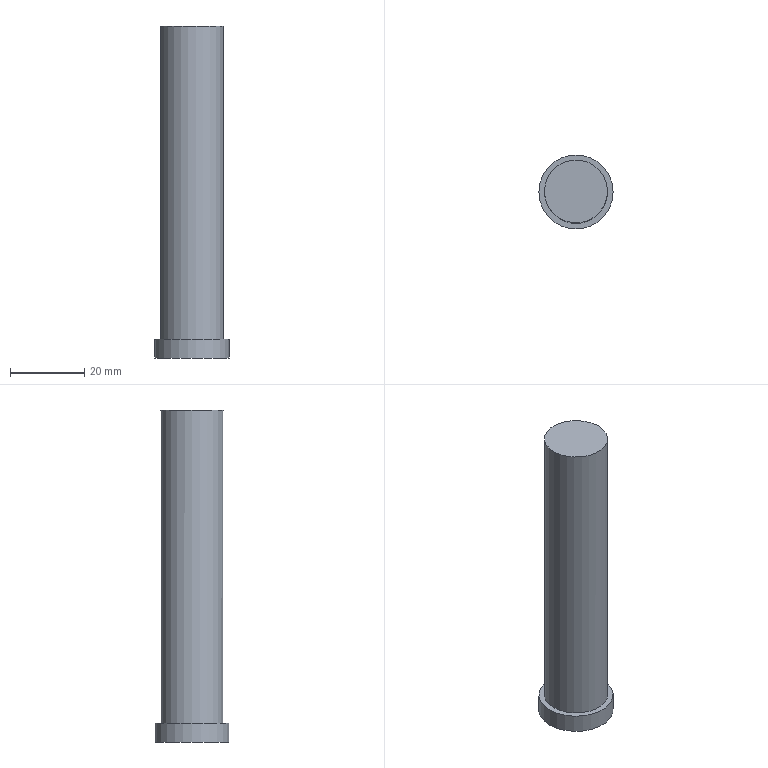Part | NX | features 23 2 | 1 solid | 5 faces | box 20 x 20 x 89.5 mm | volume 20751 mm3 | plane 3 | cylinder 2 | commonest cylinder face diameters 17 x1 20 x1
STEP:
#1=CARTESIAN_POINT('',(3000.893,49.453,-3.5));
#2=VERTEX_POINT('',#1);
#3=CARTESIAN_POINT('',(3000.,41.,-3.5));
#4=DIRECTION('',(0.,0.,1.));
#5=DIRECTION('',(1.,0.,0.));
#6=AXIS2_PLACEMENT_3D('',#3,#4,#5);
#7=CIRCLE('',#6,8.5);
#8=EDGE_CURVE('',#2,#2,#7,.T.);
#9=ORIENTED_EDGE('',*,*,#8,.F.);
#10=EDGE_LOOP('',(#9));
#11=FACE_BOUND('',#10,.T.);
#12=CARTESIAN_POINT('',(2991.5,41.,-88.));
#13=VERTEX_POINT('',#12);
#14=CARTESIAN_POINT('',(3000.,41.,-88.));
#15=DIRECTION('',(0.,0.,1.));
#16=DIRECTION('',(-1.,0.,0.));
#17=AXIS2_PLACEMENT_3D('',#14,#15,#16);
#18=CIRCLE('',#17,8.5);
#19=EDGE_CURVE('',#13,#13,#18,.T.);
#20=ORIENTED_EDGE('',*,*,#19,.T.);
#21=EDGE_LOOP('',(#20));
#22=FACE_BOUND('',#21,.T.);
#23=CARTESIAN_POINT('',(3000.,41.,-399.));
#24=DIRECTION('',(0.,0.,1.));
#25=DIRECTION('',(-1.,0.,0.));
#26=AXIS2_PLACEMENT_3D('',#23,#24,#25);
#27=CYLINDRICAL_SURFACE('',#26,8.5);
#28=ADVANCED_FACE('',(#11,#22),#27,.T.);
#29=ORIENTED_EDGE('',*,*,#8,.T.);
#30=EDGE_LOOP('',(#29));
#31=FACE_BOUND('',#30,.T.);
#32=CARTESIAN_POINT('',(3020.808,3.244,-3.5));
#33=DIRECTION('',(0.,-0.000000004,-1.));
#34=DIRECTION('',(-0.9367,0.3502,-0.000000001));
#35=AXIS2_PLACEMENT_3D('',#32,#33,#34);
#36=PLANE('',#35);
#37=ADVANCED_FACE('',(#31),#36,.F.);
#38=CARTESIAN_POINT('',(2990.,41.,-88.));
#39=VERTEX_POINT('',#38);
#40=CARTESIAN_POINT('',(3000.,41.,-88.));
#41=DIRECTION('',(0.,0.,-1.));
#42=DIRECTION('',(-1.,0.,0.));
#43=AXIS2_PLACEMENT_3D('',#40,#41,#42);
#44=CIRCLE('',#43,10.);
#45=EDGE_CURVE('',#39,#39,#44,.T.);
#46=ORIENTED_EDGE('',*,*,#45,.F.);
#47=EDGE_LOOP('',(#46));
#48=FACE_BOUND('',#47,.T.);
#49=ORIENTED_EDGE('',*,*,#19,.F.);
#50=EDGE_LOOP('',(#49));
#51=FACE_BOUND('',#50,.T.);
#52=CARTESIAN_POINT('',(3000.,41.,-88.));
#53=DIRECTION('',(0.,0.,-1.));
#54=DIRECTION('',(1.,0.,0.));
#55=AXIS2_PLACEMENT_3D('',#52,#53,#54);
#56=PLANE('',#55);
#57=ADVANCED_FACE('',(#48,#51),#56,.F.);
#58=CARTESIAN_POINT('',(2990.,41.,-93.));
#59=VERTEX_POINT('',#58);
#60=CARTESIAN_POINT('',(3000.,41.,-93.));
#61=DIRECTION('',(0.,0.,1.));
#62=DIRECTION('',(-1.,0.,0.));
#63=AXIS2_PLACEMENT_3D('',#60,#61,#62);
#64=CIRCLE('',#63,10.);
#65=EDGE_CURVE('',#59,#59,#64,.T.);
#66=ORIENTED_EDGE('',*,*,#65,.F.);
#67=EDGE_LOOP('',(#66));
#68=FACE_BOUND('',#67,.T.);
#69=CARTESIAN_POINT('',(1346.5,-267.,-93.));
#70=DIRECTION('',(0.,0.,-1.));
#71=DIRECTION('',(-1.,0.,0.));
#72=AXIS2_PLACEMENT_3D('',#69,#70,#71);
#73=PLANE('',#72);
#74=ADVANCED_FACE('',(#68),#73,.T.);
#75=ORIENTED_EDGE('',*,*,#45,.T.);
#76=EDGE_LOOP('',(#75));
#77=FACE_BOUND('',#76,.T.);
#78=ORIENTED_EDGE('',*,*,#65,.T.);
#79=EDGE_LOOP('',(#78));
#80=FACE_BOUND('',#79,.T.);
#81=CARTESIAN_POINT('',(3000.,41.,-399.));
#82=DIRECTION('',(0.,0.,1.));
#83=DIRECTION('',(-1.,0.,0.));
#84=AXIS2_PLACEMENT_3D('',#81,#82,#83);
#85=CYLINDRICAL_SURFACE('',#84,10.);
#86=ADVANCED_FACE('',(#77,#80),#85,.T.);
#87=CLOSED_SHELL('',(#28,#37,#57,#74,#86));
#88=MANIFOLD_SOLID_BREP('',#87);
#89=(LENGTH_UNIT()NAMED_UNIT(*)SI_UNIT(.MILLI.,.METRE.));
#90=UNCERTAINTY_MEASURE_WITH_UNIT(LENGTH_MEASURE(0.00001),#89,'','');
#91=(NAMED_UNIT(*)PLANE_ANGLE_UNIT()SI_UNIT($,.RADIAN.));
#92=(NAMED_UNIT(*)SI_UNIT($,.STERADIAN.)SOLID_ANGLE_UNIT());
#93=(GEOMETRIC_REPRESENTATION_CONTEXT(3)GLOBAL_UNCERTAINTY_ASSIGNED_CONTEXT((#90))GLOBAL_UNIT_ASSIGNED_CONTEXT((#89,#91,#92))REPRESENTATION_CONTEXT('',''));
#94=ADVANCED_BREP_SHAPE_REPRESENTATION('',(#88),#93);